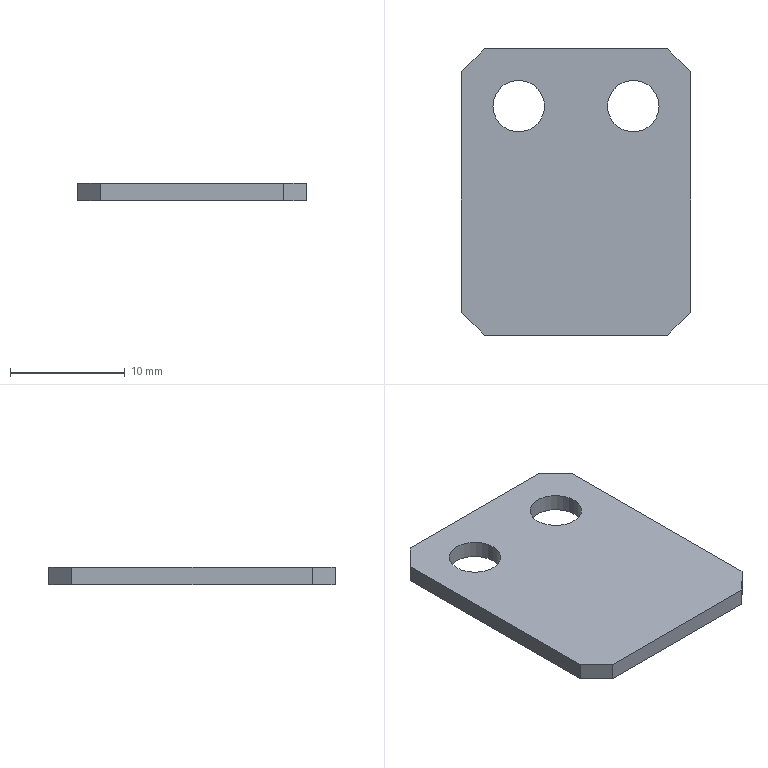Part | NX | 1 solid | 12 faces | box 20 x 25 x 1.5 mm | volume 690.287 mm3 | plane 10 | cylinder 2 | commonest cylinder face diameters 4.5 x2
STEP:
#1=CARTESIAN_POINT('',(10.,-10.5,1.5));
#2=VERTEX_POINT('',#1);
#3=CARTESIAN_POINT('',(10.,10.5,1.5));
#4=VERTEX_POINT('',#3);
#5=CARTESIAN_POINT('',(10.,12.5,1.5));
#6=DIRECTION('',(0.,1.,0.));
#7=VECTOR('',#6,1000.);
#8=LINE('',#5,#7);
#9=EDGE_CURVE('',#2,#4,#8,.T.);
#10=ORIENTED_EDGE('',*,*,#9,.F.);
#11=CARTESIAN_POINT('',(10.,-10.5,0.));
#12=VERTEX_POINT('',#11);
#13=CARTESIAN_POINT('',(10.,-10.5,1.5));
#14=DIRECTION('',(0.,0.,-1.));
#15=VECTOR('',#14,1000.);
#16=LINE('',#13,#15);
#17=EDGE_CURVE('',#2,#12,#16,.T.);
#18=ORIENTED_EDGE('',*,*,#17,.T.);
#19=CARTESIAN_POINT('',(10.,10.5,0.));
#20=VERTEX_POINT('',#19);
#21=CARTESIAN_POINT('',(10.,12.5,0.));
#22=DIRECTION('',(0.,1.,0.));
#23=VECTOR('',#22,1000.);
#24=LINE('',#21,#23);
#25=EDGE_CURVE('',#12,#20,#24,.T.);
#26=ORIENTED_EDGE('',*,*,#25,.T.);
#27=CARTESIAN_POINT('',(10.,10.5,1.5));
#28=DIRECTION('',(0.,0.,1.));
#29=VECTOR('',#28,1000.);
#30=LINE('',#27,#29);
#31=EDGE_CURVE('',#20,#4,#30,.T.);
#32=ORIENTED_EDGE('',*,*,#31,.T.);
#33=EDGE_LOOP('',(#10,#18,#26,#32));
#34=FACE_BOUND('',#33,.T.);
#35=CARTESIAN_POINT('',(10.,12.5,1.5));
#36=DIRECTION('',(-1.,0.,0.));
#37=DIRECTION('',(0.,-1.,0.));
#38=AXIS2_PLACEMENT_3D('',#35,#36,#37);
#39=PLANE('',#38);
#40=ADVANCED_FACE('',(#34),#39,.F.);
#41=CARTESIAN_POINT('',(8.,12.5,0.));
#42=VERTEX_POINT('',#41);
#43=CARTESIAN_POINT('',(-8.,12.5,0.));
#44=VERTEX_POINT('',#43);
#45=CARTESIAN_POINT('',(-10.,12.5,0.));
#46=DIRECTION('',(-1.,0.,0.));
#47=VECTOR('',#46,1000.);
#48=LINE('',#45,#47);
#49=EDGE_CURVE('',#42,#44,#48,.T.);
#50=ORIENTED_EDGE('',*,*,#49,.T.);
#51=CARTESIAN_POINT('',(-8.,12.5,1.5));
#52=VERTEX_POINT('',#51);
#53=CARTESIAN_POINT('',(-8.,12.5,1.5));
#54=DIRECTION('',(0.,0.,1.));
#55=VECTOR('',#54,1000.);
#56=LINE('',#53,#55);
#57=EDGE_CURVE('',#44,#52,#56,.T.);
#58=ORIENTED_EDGE('',*,*,#57,.T.);
#59=CARTESIAN_POINT('',(8.,12.5,1.5));
#60=VERTEX_POINT('',#59);
#61=CARTESIAN_POINT('',(-10.,12.5,1.5));
#62=DIRECTION('',(-1.,0.,0.));
#63=VECTOR('',#62,1000.);
#64=LINE('',#61,#63);
#65=EDGE_CURVE('',#60,#52,#64,.T.);
#66=ORIENTED_EDGE('',*,*,#65,.F.);
#67=CARTESIAN_POINT('',(8.,12.5,1.5));
#68=DIRECTION('',(0.,0.,-1.));
#69=VECTOR('',#68,1000.);
#70=LINE('',#67,#69);
#71=EDGE_CURVE('',#60,#42,#70,.T.);
#72=ORIENTED_EDGE('',*,*,#71,.T.);
#73=EDGE_LOOP('',(#50,#58,#66,#72));
#74=FACE_BOUND('',#73,.T.);
#75=CARTESIAN_POINT('',(-10.,12.5,1.5));
#76=DIRECTION('',(0.,-1.,0.));
#77=DIRECTION('',(0.,0.,-1.));
#78=AXIS2_PLACEMENT_3D('',#75,#76,#77);
#79=PLANE('',#78);
#80=ADVANCED_FACE('',(#74),#79,.F.);
#81=CARTESIAN_POINT('',(-10.,10.5,0.));
#82=VERTEX_POINT('',#81);
#83=CARTESIAN_POINT('',(-10.,-10.5,0.));
#84=VERTEX_POINT('',#83);
#85=CARTESIAN_POINT('',(-10.,12.5,0.));
#86=DIRECTION('',(0.,-1.,0.));
#87=VECTOR('',#86,1000.);
#88=LINE('',#85,#87);
#89=EDGE_CURVE('',#82,#84,#88,.T.);
#90=ORIENTED_EDGE('',*,*,#89,.T.);
#91=CARTESIAN_POINT('',(-10.,-10.5,1.5));
#92=VERTEX_POINT('',#91);
#93=CARTESIAN_POINT('',(-10.,-10.5,1.5));
#94=DIRECTION('',(0.,0.,1.));
#95=VECTOR('',#94,1000.);
#96=LINE('',#93,#95);
#97=EDGE_CURVE('',#84,#92,#96,.T.);
#98=ORIENTED_EDGE('',*,*,#97,.T.);
#99=CARTESIAN_POINT('',(-10.,10.5,1.5));
#100=VERTEX_POINT('',#99);
#101=CARTESIAN_POINT('',(-10.,12.5,1.5));
#102=DIRECTION('',(0.,-1.,0.));
#103=VECTOR('',#102,1000.);
#104=LINE('',#101,#103);
#105=EDGE_CURVE('',#100,#92,#104,.T.);
#106=ORIENTED_EDGE('',*,*,#105,.F.);
#107=CARTESIAN_POINT('',(-10.,10.5,1.5));
#108=DIRECTION('',(0.,0.,-1.));
#109=VECTOR('',#108,1000.);
#110=LINE('',#107,#109);
#111=EDGE_CURVE('',#100,#82,#110,.T.);
#112=ORIENTED_EDGE('',*,*,#111,.T.);
#113=EDGE_LOOP('',(#90,#98,#106,#112));
#114=FACE_BOUND('',#113,.T.);
#115=CARTESIAN_POINT('',(-10.,12.5,1.5));
#116=DIRECTION('',(1.,0.,0.));
#117=DIRECTION('',(0.,1.,0.));
#118=AXIS2_PLACEMENT_3D('',#115,#116,#117);
#119=PLANE('',#118);
#120=ADVANCED_FACE('',(#114),#119,.F.);
#121=CARTESIAN_POINT('',(-8.,-12.5,0.));
#122=VERTEX_POINT('',#121);
#123=CARTESIAN_POINT('',(8.,-12.5,0.));
#124=VERTEX_POINT('',#123);
#125=CARTESIAN_POINT('',(-10.,-12.5,0.));
#126=DIRECTION('',(1.,0.,0.));
#127=VECTOR('',#126,1000.);
#128=LINE('',#125,#127);
#129=EDGE_CURVE('',#122,#124,#128,.T.);
#130=ORIENTED_EDGE('',*,*,#129,.T.);
#131=CARTESIAN_POINT('',(8.,-12.5,1.5));
#132=VERTEX_POINT('',#131);
#133=CARTESIAN_POINT('',(8.,-12.5,1.5));
#134=DIRECTION('',(0.,0.,1.));
#135=VECTOR('',#134,1000.);
#136=LINE('',#133,#135);
#137=EDGE_CURVE('',#124,#132,#136,.T.);
#138=ORIENTED_EDGE('',*,*,#137,.T.);
#139=CARTESIAN_POINT('',(-8.,-12.5,1.5));
#140=VERTEX_POINT('',#139);
#141=CARTESIAN_POINT('',(-10.,-12.5,1.5));
#142=DIRECTION('',(1.,0.,0.));
#143=VECTOR('',#142,1000.);
#144=LINE('',#141,#143);
#145=EDGE_CURVE('',#140,#132,#144,.T.);
#146=ORIENTED_EDGE('',*,*,#145,.F.);
#147=CARTESIAN_POINT('',(-8.,-12.5,1.5));
#148=DIRECTION('',(0.,0.,-1.));
#149=VECTOR('',#148,1000.);
#150=LINE('',#147,#149);
#151=EDGE_CURVE('',#140,#122,#150,.T.);
#152=ORIENTED_EDGE('',*,*,#151,.T.);
#153=EDGE_LOOP('',(#130,#138,#146,#152));
#154=FACE_BOUND('',#153,.T.);
#155=CARTESIAN_POINT('',(-10.,-12.5,1.5));
#156=DIRECTION('',(0.,1.,0.));
#157=DIRECTION('',(0.,0.,1.));
#158=AXIS2_PLACEMENT_3D('',#155,#156,#157);
#159=PLANE('',#158);
#160=ADVANCED_FACE('',(#154),#159,.F.);
#161=CARTESIAN_POINT('',(-2.75,7.5,1.5));
#162=VERTEX_POINT('',#161);
#163=CARTESIAN_POINT('',(-5.,7.5,1.5));
#164=DIRECTION('',(0.,0.,1.));
#165=DIRECTION('',(1.,0.,0.));
#166=AXIS2_PLACEMENT_3D('',#163,#164,#165);
#167=CIRCLE('',#166,2.25);
#168=EDGE_CURVE('',#162,#162,#167,.T.);
#169=ORIENTED_EDGE('',*,*,#168,.F.);
#170=EDGE_LOOP('',(#169));
#171=FACE_BOUND('',#170,.T.);
#172=CARTESIAN_POINT('',(7.25,7.5,1.5));
#173=VERTEX_POINT('',#172);
#174=CARTESIAN_POINT('',(5.,7.5,1.5));
#175=DIRECTION('',(0.,0.,1.));
#176=DIRECTION('',(1.,0.,0.));
#177=AXIS2_PLACEMENT_3D('',#174,#175,#176);
#178=CIRCLE('',#177,2.25);
#179=EDGE_CURVE('',#173,#173,#178,.T.);
#180=ORIENTED_EDGE('',*,*,#179,.F.);
#181=EDGE_LOOP('',(#180));
#182=FACE_BOUND('',#181,.T.);
#183=ORIENTED_EDGE('',*,*,#145,.T.);
#184=CARTESIAN_POINT('',(10.25,-10.25,1.5));
#185=DIRECTION('',(-0.7071,-0.7071,0.));
#186=VECTOR('',#185,1000.);
#187=LINE('',#184,#186);
#188=EDGE_CURVE('',#132,#2,#187,.F.);
#189=ORIENTED_EDGE('',*,*,#188,.T.);
#190=ORIENTED_EDGE('',*,*,#9,.T.);
#191=CARTESIAN_POINT('',(10.25,10.25,1.5));
#192=DIRECTION('',(0.7071,-0.7071,0.));
#193=VECTOR('',#192,1000.);
#194=LINE('',#191,#193);
#195=EDGE_CURVE('',#4,#60,#194,.F.);
#196=ORIENTED_EDGE('',*,*,#195,.T.);
#197=ORIENTED_EDGE('',*,*,#65,.T.);
#198=CARTESIAN_POINT('',(-10.25,10.25,1.5));
#199=DIRECTION('',(0.7071,0.7071,0.));
#200=VECTOR('',#199,1000.);
#201=LINE('',#198,#200);
#202=EDGE_CURVE('',#52,#100,#201,.F.);
#203=ORIENTED_EDGE('',*,*,#202,.T.);
#204=ORIENTED_EDGE('',*,*,#105,.T.);
#205=CARTESIAN_POINT('',(-10.25,-10.25,1.5));
#206=DIRECTION('',(-0.7071,0.7071,0.));
#207=VECTOR('',#206,1000.);
#208=LINE('',#205,#207);
#209=EDGE_CURVE('',#92,#140,#208,.F.);
#210=ORIENTED_EDGE('',*,*,#209,.T.);
#211=EDGE_LOOP('',(#183,#189,#190,#196,#197,#203,#204,#210));
#212=FACE_BOUND('',#211,.T.);
#213=CARTESIAN_POINT('',(0.,0.,1.5));
#214=DIRECTION('',(0.,0.,1.));
#215=DIRECTION('',(1.,0.,0.));
#216=AXIS2_PLACEMENT_3D('',#213,#214,#215);
#217=PLANE('',#216);
#218=ADVANCED_FACE('',(#171,#182,#212),#217,.T.);
#219=CARTESIAN_POINT('',(-2.75,7.5,0.));
#220=VERTEX_POINT('',#219);
#221=CARTESIAN_POINT('',(-5.,7.5,0.));
#222=DIRECTION('',(0.,0.,1.));
#223=DIRECTION('',(1.,0.,0.));
#224=AXIS2_PLACEMENT_3D('',#221,#222,#223);
#225=CIRCLE('',#224,2.25);
#226=EDGE_CURVE('',#220,#220,#225,.T.);
#227=ORIENTED_EDGE('',*,*,#226,.T.);
#228=EDGE_LOOP('',(#227));
#229=FACE_BOUND('',#228,.T.);
#230=CARTESIAN_POINT('',(7.25,7.5,0.));
#231=VERTEX_POINT('',#230);
#232=CARTESIAN_POINT('',(5.,7.5,0.));
#233=DIRECTION('',(0.,0.,1.));
#234=DIRECTION('',(1.,0.,0.));
#235=AXIS2_PLACEMENT_3D('',#232,#233,#234);
#236=CIRCLE('',#235,2.25);
#237=EDGE_CURVE('',#231,#231,#236,.T.);
#238=ORIENTED_EDGE('',*,*,#237,.T.);
#239=EDGE_LOOP('',(#238));
#240=FACE_BOUND('',#239,.T.);
#241=ORIENTED_EDGE('',*,*,#25,.F.);
#242=CARTESIAN_POINT('',(10.,-10.5,0.));
#243=DIRECTION('',(0.7071,0.7071,0.));
#244=VECTOR('',#243,1000.);
#245=LINE('',#242,#244);
#246=EDGE_CURVE('',#12,#124,#245,.F.);
#247=ORIENTED_EDGE('',*,*,#246,.T.);
#248=ORIENTED_EDGE('',*,*,#129,.F.);
#249=CARTESIAN_POINT('',(-8.,-12.5,0.));
#250=DIRECTION('',(0.7071,-0.7071,0.));
#251=VECTOR('',#250,1000.);
#252=LINE('',#249,#251);
#253=EDGE_CURVE('',#122,#84,#252,.F.);
#254=ORIENTED_EDGE('',*,*,#253,.T.);
#255=ORIENTED_EDGE('',*,*,#89,.F.);
#256=CARTESIAN_POINT('',(-10.,10.5,0.));
#257=DIRECTION('',(-0.7071,-0.7071,0.));
#258=VECTOR('',#257,1000.);
#259=LINE('',#256,#258);
#260=EDGE_CURVE('',#82,#44,#259,.F.);
#261=ORIENTED_EDGE('',*,*,#260,.T.);
#262=ORIENTED_EDGE('',*,*,#49,.F.);
#263=CARTESIAN_POINT('',(8.,12.5,0.));
#264=DIRECTION('',(-0.7071,0.7071,0.));
#265=VECTOR('',#264,1000.);
#266=LINE('',#263,#265);
#267=EDGE_CURVE('',#42,#20,#266,.F.);
#268=ORIENTED_EDGE('',*,*,#267,.T.);
#269=EDGE_LOOP('',(#241,#247,#248,#254,#255,#261,#262,#268));
#270=FACE_BOUND('',#269,.T.);
#271=CARTESIAN_POINT('',(0.,0.,0.));
#272=DIRECTION('',(0.,0.,1.));
#273=DIRECTION('',(1.,0.,0.));
#274=AXIS2_PLACEMENT_3D('',#271,#272,#273);
#275=PLANE('',#274);
#276=ADVANCED_FACE('',(#229,#240,#270),#275,.F.);
#277=ORIENTED_EDGE('',*,*,#179,.T.);
#278=EDGE_LOOP('',(#277));
#279=FACE_BOUND('',#278,.T.);
#280=ORIENTED_EDGE('',*,*,#237,.F.);
#281=EDGE_LOOP('',(#280));
#282=FACE_BOUND('',#281,.T.);
#283=CARTESIAN_POINT('',(5.,7.5,1.5));
#284=DIRECTION('',(0.,0.,1.));
#285=DIRECTION('',(1.,0.,0.));
#286=AXIS2_PLACEMENT_3D('',#283,#284,#285);
#287=CYLINDRICAL_SURFACE('',#286,2.25);
#288=ADVANCED_FACE('',(#279,#282),#287,.F.);
#289=ORIENTED_EDGE('',*,*,#168,.T.);
#290=EDGE_LOOP('',(#289));
#291=FACE_BOUND('',#290,.T.);
#292=ORIENTED_EDGE('',*,*,#226,.F.);
#293=EDGE_LOOP('',(#292));
#294=FACE_BOUND('',#293,.T.);
#295=CARTESIAN_POINT('',(-5.,7.5,1.5));
#296=DIRECTION('',(0.,0.,1.));
#297=DIRECTION('',(1.,0.,0.));
#298=AXIS2_PLACEMENT_3D('',#295,#296,#297);
#299=CYLINDRICAL_SURFACE('',#298,2.25);
#300=ADVANCED_FACE('',(#291,#294),#299,.F.);
#301=ORIENTED_EDGE('',*,*,#188,.F.);
#302=ORIENTED_EDGE('',*,*,#137,.F.);
#303=ORIENTED_EDGE('',*,*,#246,.F.);
#304=ORIENTED_EDGE('',*,*,#17,.F.);
#305=EDGE_LOOP('',(#301,#302,#303,#304));
#306=FACE_BOUND('',#305,.T.);
#307=CARTESIAN_POINT('',(10.,-10.5,1.5));
#308=DIRECTION('',(-0.7071,0.7071,0.));
#309=DIRECTION('',(0.,0.,-1.));
#310=AXIS2_PLACEMENT_3D('',#307,#308,#309);
#311=PLANE('',#310);
#312=ADVANCED_FACE('',(#306),#311,.F.);
#313=ORIENTED_EDGE('',*,*,#209,.F.);
#314=ORIENTED_EDGE('',*,*,#97,.F.);
#315=ORIENTED_EDGE('',*,*,#253,.F.);
#316=ORIENTED_EDGE('',*,*,#151,.F.);
#317=EDGE_LOOP('',(#313,#314,#315,#316));
#318=FACE_BOUND('',#317,.T.);
#319=CARTESIAN_POINT('',(-8.,-12.5,1.5));
#320=DIRECTION('',(0.7071,0.7071,0.));
#321=DIRECTION('',(0.,0.,-1.));
#322=AXIS2_PLACEMENT_3D('',#319,#320,#321);
#323=PLANE('',#322);
#324=ADVANCED_FACE('',(#318),#323,.F.);
#325=ORIENTED_EDGE('',*,*,#202,.F.);
#326=ORIENTED_EDGE('',*,*,#57,.F.);
#327=ORIENTED_EDGE('',*,*,#260,.F.);
#328=ORIENTED_EDGE('',*,*,#111,.F.);
#329=EDGE_LOOP('',(#325,#326,#327,#328));
#330=FACE_BOUND('',#329,.T.);
#331=CARTESIAN_POINT('',(-10.,10.5,1.5));
#332=DIRECTION('',(0.7071,-0.7071,0.));
#333=DIRECTION('',(0.,0.,-1.));
#334=AXIS2_PLACEMENT_3D('',#331,#332,#333);
#335=PLANE('',#334);
#336=ADVANCED_FACE('',(#330),#335,.F.);
#337=ORIENTED_EDGE('',*,*,#195,.F.);
#338=ORIENTED_EDGE('',*,*,#31,.F.);
#339=ORIENTED_EDGE('',*,*,#267,.F.);
#340=ORIENTED_EDGE('',*,*,#71,.F.);
#341=EDGE_LOOP('',(#337,#338,#339,#340));
#342=FACE_BOUND('',#341,.T.);
#343=CARTESIAN_POINT('',(8.,12.5,1.5));
#344=DIRECTION('',(-0.7071,-0.7071,0.));
#345=DIRECTION('',(0.,0.,-1.));
#346=AXIS2_PLACEMENT_3D('',#343,#344,#345);
#347=PLANE('',#346);
#348=ADVANCED_FACE('',(#342),#347,.F.);
#349=CLOSED_SHELL('',(#40,#80,#120,#160,#218,#276,#288,#300,#312,#324,#336,#348));
#350=MANIFOLD_SOLID_BREP('',#349);
#351=(LENGTH_UNIT()NAMED_UNIT(*)SI_UNIT(.MILLI.,.METRE.));
#352=UNCERTAINTY_MEASURE_WITH_UNIT(LENGTH_MEASURE(0.00001),#351,'','');
#353=(NAMED_UNIT(*)PLANE_ANGLE_UNIT()SI_UNIT($,.RADIAN.));
#354=(NAMED_UNIT(*)SI_UNIT($,.STERADIAN.)SOLID_ANGLE_UNIT());
#355=(GEOMETRIC_REPRESENTATION_CONTEXT(3)GLOBAL_UNCERTAINTY_ASSIGNED_CONTEXT((#352))GLOBAL_UNIT_ASSIGNED_CONTEXT((#351,#353,#354))REPRESENTATION_CONTEXT('',''));
#356=ADVANCED_BREP_SHAPE_REPRESENTATION('',(#350),#355);